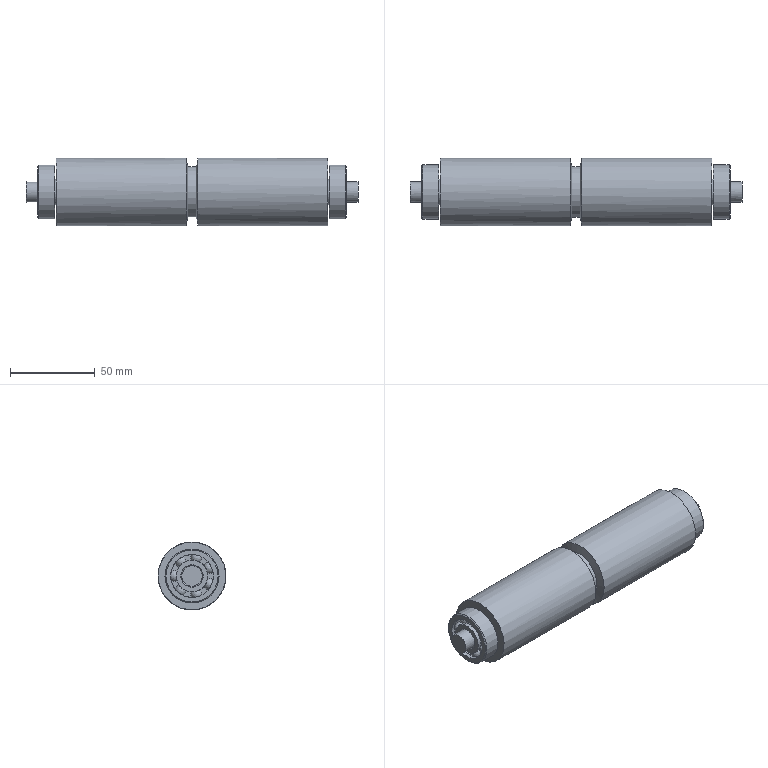Part | STEP file | YBQDJ-SSJ-6 | 1 solid | 85 faces | box 196 x 40 x 40 mm | volume 211425 mm3 | torus 28 | cylinder 17 | plane 14 | sphere 14 | cone 12 | commonest cylinder face diameters 12 x4 18.667 x4 15 x2 25.333 x2 32 x2 40 x2